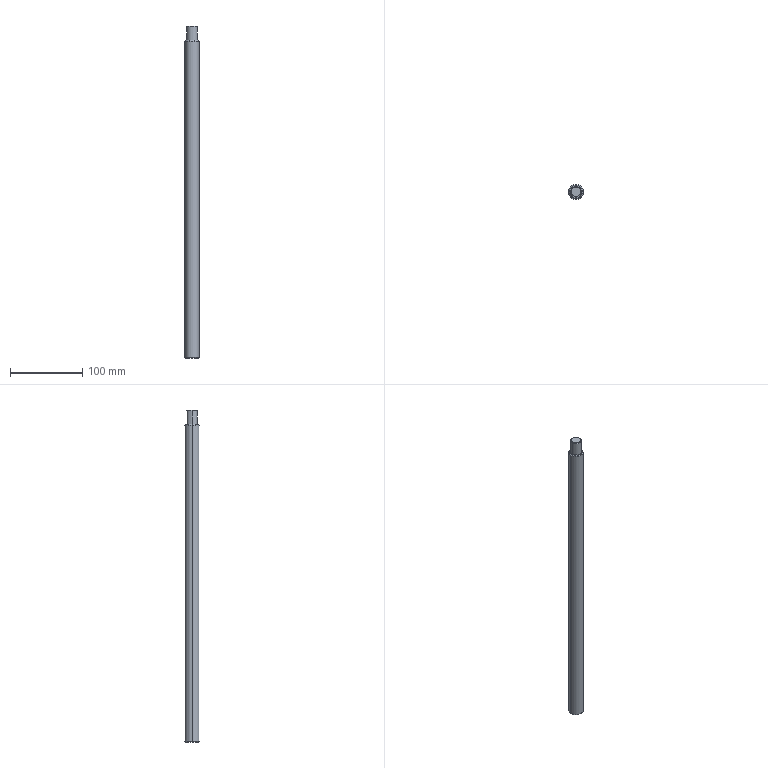Part | STEP file | 1 solid | 13 faces | box 20 x 20 x 460 mm | volume 141681 mm3 | cone 6 | cylinder 4 | plane 3 | commonest cylinder face diameters 15 x2 20 x2
STEP:
#1=CARTESIAN_POINT('',(0.,0.,0.));
#2=DIRECTION('',(0.,0.,1.));
#3=DIRECTION('',(1.,0.,0.));
#4=AXIS2_PLACEMENT_3D('',#1,#2,#3);
#5=CARTESIAN_POINT('',(10.,0.,-229.));
#6=VERTEX_POINT('',#5);
#7=CARTESIAN_POINT('',(-10.,0.,-229.));
#8=VERTEX_POINT('',#7);
#9=CARTESIAN_POINT('',(0.,0.,-229.));
#10=DIRECTION('',(0.,0.,1.));
#11=DIRECTION('',(1.,0.,0.));
#12=AXIS2_PLACEMENT_3D('',#9,#10,#11);
#13=CIRCLE('',#12,10.);
#14=CARTESIAN_POINT('',(0.,0.,230.));
#15=DIRECTION('',(0.,0.,1.));
#16=DIRECTION('',(1.,0.,0.));
#17=AXIS2_PLACEMENT_3D('',#14,#15,#16);
#18=CYLINDRICAL_SURFACE('',#17,10.);
#19=CARTESIAN_POINT('',(0.,-459.));
#20=DIRECTION('',(1.,0.));
#21=VECTOR('',#20,1.);
#22=LINE('',#19,#21);
#23=(GEOMETRIC_REPRESENTATION_CONTEXT(2)PARAMETRIC_REPRESENTATION_CONTEXT()REPRESENTATION_CONTEXT('',''));
#24=DEFINITIONAL_REPRESENTATION('',(#22),#23);
#25=PCURVE('',#18,#24);
#26=CARTESIAN_POINT('',(0.,0.,-229.));
#27=DIRECTION('',(0.,0.,1.));
#28=DIRECTION('',(1.,0.,0.));
#29=AXIS2_PLACEMENT_3D('',#26,#27,#28);
#30=CONICAL_SURFACE('',#29,10.,0.7854);
#31=CARTESIAN_POINT('',(0.,0.));
#32=DIRECTION('',(1.,0.));
#33=VECTOR('',#32,1.);
#34=LINE('',#31,#33);
#35=(GEOMETRIC_REPRESENTATION_CONTEXT(2)PARAMETRIC_REPRESENTATION_CONTEXT()REPRESENTATION_CONTEXT('',''));
#36=DEFINITIONAL_REPRESENTATION('',(#34),#35);
#37=PCURVE('',#30,#36);
#38=SURFACE_CURVE('',#13,(#25,#37),.PCURVE_S1.);
#39=EDGE_CURVE('',#6,#8,#38,.T.);
#40=ORIENTED_EDGE('',*,*,#39,.T.);
#41=CARTESIAN_POINT('',(-10.,0.,209.));
#42=VERTEX_POINT('',#41);
#43=CARTESIAN_POINT('',(-10.,0.,230.));
#44=DIRECTION('',(0.,0.,1.));
#45=VECTOR('',#44,1.);
#46=LINE('',#43,#45);
#47=CARTESIAN_POINT('',(3.142,0.));
#48=DIRECTION('',(0.,1.));
#49=VECTOR('',#48,1.);
#50=LINE('',#47,#49);
#51=(GEOMETRIC_REPRESENTATION_CONTEXT(2)PARAMETRIC_REPRESENTATION_CONTEXT()REPRESENTATION_CONTEXT('',''));
#52=DEFINITIONAL_REPRESENTATION('',(#50),#51);
#53=PCURVE('',#18,#52);
#54=CARTESIAN_POINT('',(0.,0.,230.));
#55=DIRECTION('',(0.,0.,1.));
#56=DIRECTION('',(1.,0.,0.));
#57=AXIS2_PLACEMENT_3D('',#54,#55,#56);
#58=CYLINDRICAL_SURFACE('',#57,10.);
#59=CARTESIAN_POINT('',(3.142,0.));
#60=DIRECTION('',(0.,1.));
#61=VECTOR('',#60,1.);
#62=LINE('',#59,#61);
#63=(GEOMETRIC_REPRESENTATION_CONTEXT(2)PARAMETRIC_REPRESENTATION_CONTEXT()REPRESENTATION_CONTEXT('',''));
#64=DEFINITIONAL_REPRESENTATION('',(#62),#63);
#65=PCURVE('',#58,#64);
#66=SURFACE_CURVE('',#46,(#53,#65),.PCURVE_S1.);
#67=EDGE_CURVE('',#8,#42,#66,.T.);
#68=ORIENTED_EDGE('',*,*,#67,.T.);
#69=CARTESIAN_POINT('',(10.,0.,209.));
#70=VERTEX_POINT('',#69);
#71=CARTESIAN_POINT('',(0.,0.,209.));
#72=DIRECTION('',(0.,0.,-1.));
#73=DIRECTION('',(1.,0.,0.));
#74=AXIS2_PLACEMENT_3D('',#71,#72,#73);
#75=CIRCLE('',#74,10.);
#76=CARTESIAN_POINT('',(6.283,-21.));
#77=DIRECTION('',(-1.,0.));
#78=VECTOR('',#77,1.);
#79=LINE('',#76,#78);
#80=(GEOMETRIC_REPRESENTATION_CONTEXT(2)PARAMETRIC_REPRESENTATION_CONTEXT()REPRESENTATION_CONTEXT('',''));
#81=DEFINITIONAL_REPRESENTATION('',(#79),#80);
#82=PCURVE('',#18,#81);
#83=CARTESIAN_POINT('',(0.,0.,209.));
#84=DIRECTION('',(0.,0.,-1.));
#85=DIRECTION('',(-1.,0.,0.));
#86=AXIS2_PLACEMENT_3D('',#83,#84,#85);
#87=CONICAL_SURFACE('',#86,10.,0.7854);
#88=CARTESIAN_POINT('',(-3.142,0.));
#89=DIRECTION('',(1.,0.));
#90=VECTOR('',#89,1.);
#91=LINE('',#88,#90);
#92=(GEOMETRIC_REPRESENTATION_CONTEXT(2)PARAMETRIC_REPRESENTATION_CONTEXT()REPRESENTATION_CONTEXT('',''));
#93=DEFINITIONAL_REPRESENTATION('',(#91),#92);
#94=PCURVE('',#87,#93);
#95=SURFACE_CURVE('',#75,(#82,#94),.PCURVE_S1.);
#96=EDGE_CURVE('',#42,#70,#95,.T.);
#97=ORIENTED_EDGE('',*,*,#96,.T.);
#98=CARTESIAN_POINT('',(10.,0.,230.));
#99=DIRECTION('',(0.,0.,1.));
#100=VECTOR('',#99,1.);
#101=LINE('',#98,#100);
#102=CARTESIAN_POINT('',(0.,0.));
#103=DIRECTION('',(0.,1.));
#104=VECTOR('',#103,1.);
#105=LINE('',#102,#104);
#106=(GEOMETRIC_REPRESENTATION_CONTEXT(2)PARAMETRIC_REPRESENTATION_CONTEXT()REPRESENTATION_CONTEXT('',''));
#107=DEFINITIONAL_REPRESENTATION('',(#105),#106);
#108=PCURVE('',#18,#107);
#109=CARTESIAN_POINT('',(6.283,0.));
#110=DIRECTION('',(0.,1.));
#111=VECTOR('',#110,1.);
#112=LINE('',#109,#111);
#113=(GEOMETRIC_REPRESENTATION_CONTEXT(2)PARAMETRIC_REPRESENTATION_CONTEXT()REPRESENTATION_CONTEXT('',''));
#114=DEFINITIONAL_REPRESENTATION('',(#112),#113);
#115=PCURVE('',#58,#114);
#116=SURFACE_CURVE('',#101,(#108,#115),.PCURVE_S1.);
#117=EDGE_CURVE('',#6,#70,#116,.T.);
#118=ORIENTED_EDGE('',*,*,#117,.F.);
#119=EDGE_LOOP('',(#40,#68,#97,#118));
#120=FACE_BOUND('',#119,.T.);
#121=ADVANCED_FACE('',(#120),#18,.T.);
#122=CARTESIAN_POINT('',(9.,0.,-230.));
#123=VERTEX_POINT('',#122);
#124=CARTESIAN_POINT('',(-9.,0.,-230.));
#125=VERTEX_POINT('',#124);
#126=CARTESIAN_POINT('',(0.,0.,-230.));
#127=DIRECTION('',(0.,0.,1.));
#128=DIRECTION('',(1.,0.,0.));
#129=AXIS2_PLACEMENT_3D('',#126,#127,#128);
#130=CIRCLE('',#129,9.);
#131=CARTESIAN_POINT('',(0.,-1.));
#132=DIRECTION('',(1.,0.));
#133=VECTOR('',#132,1.);
#134=LINE('',#131,#133);
#135=(GEOMETRIC_REPRESENTATION_CONTEXT(2)PARAMETRIC_REPRESENTATION_CONTEXT()REPRESENTATION_CONTEXT('',''));
#136=DEFINITIONAL_REPRESENTATION('',(#134),#135);
#137=PCURVE('',#30,#136);
#138=CARTESIAN_POINT('',(0.,0.,-230.));
#139=DIRECTION('',(0.,0.,1.));
#140=DIRECTION('',(1.,0.,0.));
#141=AXIS2_PLACEMENT_3D('',#138,#139,#140);
#142=PLANE('',#141);
#143=CARTESIAN_POINT('',(0.,0.));
#144=DIRECTION('',(1.,0.));
#145=AXIS2_PLACEMENT_2D('',#143,#144);
#146=CIRCLE('',#145,9.);
#147=(GEOMETRIC_REPRESENTATION_CONTEXT(2)PARAMETRIC_REPRESENTATION_CONTEXT()REPRESENTATION_CONTEXT('',''));
#148=DEFINITIONAL_REPRESENTATION('',(#146),#147);
#149=PCURVE('',#142,#148);
#150=SURFACE_CURVE('',#130,(#137,#149),.PCURVE_S1.);
#151=EDGE_CURVE('',#123,#125,#150,.T.);
#152=ORIENTED_EDGE('',*,*,#151,.T.);
#153=CARTESIAN_POINT('',(-10.,0.,-229.));
#154=DIRECTION('',(-0.7071,0.,0.7071));
#155=VECTOR('',#154,1.);
#156=LINE('',#153,#155);
#157=CARTESIAN_POINT('',(3.142,0.));
#158=DIRECTION('',(0.,1.));
#159=VECTOR('',#158,1.);
#160=LINE('',#157,#159);
#161=(GEOMETRIC_REPRESENTATION_CONTEXT(2)PARAMETRIC_REPRESENTATION_CONTEXT()REPRESENTATION_CONTEXT('',''));
#162=DEFINITIONAL_REPRESENTATION('',(#160),#161);
#163=PCURVE('',#30,#162);
#164=CARTESIAN_POINT('',(0.,0.,-229.));
#165=DIRECTION('',(0.,0.,1.));
#166=DIRECTION('',(1.,0.,0.));
#167=AXIS2_PLACEMENT_3D('',#164,#165,#166);
#168=CONICAL_SURFACE('',#167,10.,0.7854);
#169=CARTESIAN_POINT('',(3.142,0.));
#170=DIRECTION('',(0.,1.));
#171=VECTOR('',#170,1.);
#172=LINE('',#169,#171);
#173=(GEOMETRIC_REPRESENTATION_CONTEXT(2)PARAMETRIC_REPRESENTATION_CONTEXT()REPRESENTATION_CONTEXT('',''));
#174=DEFINITIONAL_REPRESENTATION('',(#172),#173);
#175=PCURVE('',#168,#174);
#176=SURFACE_CURVE('',#156,(#163,#175),.PCURVE_S1.);
#177=EDGE_CURVE('',#125,#8,#176,.T.);
#178=ORIENTED_EDGE('',*,*,#177,.T.);
#179=ORIENTED_EDGE('',*,*,#39,.F.);
#180=CARTESIAN_POINT('',(10.,0.,-229.));
#181=DIRECTION('',(0.7071,0.,0.7071));
#182=VECTOR('',#181,1.);
#183=LINE('',#180,#182);
#184=CARTESIAN_POINT('',(0.,0.));
#185=DIRECTION('',(0.,1.));
#186=VECTOR('',#185,1.);
#187=LINE('',#184,#186);
#188=(GEOMETRIC_REPRESENTATION_CONTEXT(2)PARAMETRIC_REPRESENTATION_CONTEXT()REPRESENTATION_CONTEXT('',''));
#189=DEFINITIONAL_REPRESENTATION('',(#187),#188);
#190=PCURVE('',#30,#189);
#191=CARTESIAN_POINT('',(6.283,0.));
#192=DIRECTION('',(0.,1.));
#193=VECTOR('',#192,1.);
#194=LINE('',#191,#193);
#195=(GEOMETRIC_REPRESENTATION_CONTEXT(2)PARAMETRIC_REPRESENTATION_CONTEXT()REPRESENTATION_CONTEXT('',''));
#196=DEFINITIONAL_REPRESENTATION('',(#194),#195);
#197=PCURVE('',#168,#196);
#198=SURFACE_CURVE('',#183,(#190,#197),.PCURVE_S1.);
#199=EDGE_CURVE('',#123,#6,#198,.T.);
#200=ORIENTED_EDGE('',*,*,#199,.F.);
#201=EDGE_LOOP('',(#152,#178,#179,#200));
#202=FACE_BOUND('',#201,.T.);
#203=ADVANCED_FACE('',(#202),#30,.T.);
#204=CARTESIAN_POINT('',(-9.,0.,210.));
#205=VERTEX_POINT('',#204);
#206=CARTESIAN_POINT('',(9.,0.,210.));
#207=VERTEX_POINT('',#206);
#208=CARTESIAN_POINT('',(0.,0.,210.));
#209=DIRECTION('',(0.,0.,-1.));
#210=DIRECTION('',(-1.,0.,0.));
#211=AXIS2_PLACEMENT_3D('',#208,#209,#210);
#212=CIRCLE('',#211,9.);
#213=CARTESIAN_POINT('',(0.,-1.));
#214=DIRECTION('',(1.,0.));
#215=VECTOR('',#214,1.);
#216=LINE('',#213,#215);
#217=(GEOMETRIC_REPRESENTATION_CONTEXT(2)PARAMETRIC_REPRESENTATION_CONTEXT()REPRESENTATION_CONTEXT('',''));
#218=DEFINITIONAL_REPRESENTATION('',(#216),#217);
#219=PCURVE('',#87,#218);
#220=CARTESIAN_POINT('',(0.,0.,210.));
#221=DIRECTION('',(0.,0.,1.));
#222=DIRECTION('',(1.,0.,0.));
#223=AXIS2_PLACEMENT_3D('',#220,#221,#222);
#224=PLANE('',#223);
#225=CARTESIAN_POINT('',(-9.,0.));
#226=CARTESIAN_POINT('',(-9.,15.588));
#227=CARTESIAN_POINT('',(4.5,7.794));
#228=CARTESIAN_POINT('',(18.,0.));
#229=CARTESIAN_POINT('',(4.5,-7.794));
#230=CARTESIAN_POINT('',(-9.,-15.588));
#231=CARTESIAN_POINT('',(-9.,0.));
#232=(BOUNDED_CURVE()B_SPLINE_CURVE(2,(#225,#226,#227,#228,#229,#230,#231),.UNSPECIFIED.,.T.,.F.)B_SPLINE_CURVE_WITH_KNOTS((1,2,2,2,2,1),(-2.094,0.,2.094,4.189,6.283,8.378),.UNSPECIFIED.)CURVE()GEOMETRIC_REPRESENTATION_ITEM()RATIONAL_B_SPLINE_CURVE((1.,0.5,1.,0.5,1.,0.5,1.))REPRESENTATION_ITEM(''));
#233=(GEOMETRIC_REPRESENTATION_CONTEXT(2)PARAMETRIC_REPRESENTATION_CONTEXT()REPRESENTATION_CONTEXT('',''));
#234=DEFINITIONAL_REPRESENTATION('',(#232),#233);
#235=PCURVE('',#224,#234);
#236=SURFACE_CURVE('',#212,(#219,#235),.PCURVE_S1.);
#237=EDGE_CURVE('',#205,#207,#236,.T.);
#238=ORIENTED_EDGE('',*,*,#237,.T.);
#239=CARTESIAN_POINT('',(10.,0.,209.));
#240=DIRECTION('',(0.7071,0.,-0.7071));
#241=VECTOR('',#240,1.);
#242=LINE('',#239,#241);
#243=CARTESIAN_POINT('',(3.142,0.));
#244=DIRECTION('',(0.,1.));
#245=VECTOR('',#244,1.);
#246=LINE('',#243,#245);
#247=(GEOMETRIC_REPRESENTATION_CONTEXT(2)PARAMETRIC_REPRESENTATION_CONTEXT()REPRESENTATION_CONTEXT('',''));
#248=DEFINITIONAL_REPRESENTATION('',(#246),#247);
#249=PCURVE('',#87,#248);
#250=CARTESIAN_POINT('',(0.,0.,209.));
#251=DIRECTION('',(0.,0.,-1.));
#252=DIRECTION('',(-1.,0.,0.));
#253=AXIS2_PLACEMENT_3D('',#250,#251,#252);
#254=CONICAL_SURFACE('',#253,10.,0.7854);
#255=CARTESIAN_POINT('',(3.142,0.));
#256=DIRECTION('',(0.,1.));
#257=VECTOR('',#256,1.);
#258=LINE('',#255,#257);
#259=(GEOMETRIC_REPRESENTATION_CONTEXT(2)PARAMETRIC_REPRESENTATION_CONTEXT()REPRESENTATION_CONTEXT('',''));
#260=DEFINITIONAL_REPRESENTATION('',(#258),#259);
#261=PCURVE('',#254,#260);
#262=SURFACE_CURVE('',#242,(#249,#261),.PCURVE_S1.);
#263=EDGE_CURVE('',#207,#70,#262,.T.);
#264=ORIENTED_EDGE('',*,*,#263,.T.);
#265=ORIENTED_EDGE('',*,*,#96,.F.);
#266=CARTESIAN_POINT('',(-10.,0.,209.));
#267=DIRECTION('',(-0.7071,0.,-0.7071));
#268=VECTOR('',#267,1.);
#269=LINE('',#266,#268);
#270=CARTESIAN_POINT('',(0.,0.));
#271=DIRECTION('',(0.,1.));
#272=VECTOR('',#271,1.);
#273=LINE('',#270,#272);
#274=(GEOMETRIC_REPRESENTATION_CONTEXT(2)PARAMETRIC_REPRESENTATION_CONTEXT()REPRESENTATION_CONTEXT('',''));
#275=DEFINITIONAL_REPRESENTATION('',(#273),#274);
#276=PCURVE('',#87,#275);
#277=CARTESIAN_POINT('',(6.283,0.));
#278=DIRECTION('',(0.,1.));
#279=VECTOR('',#278,1.);
#280=LINE('',#277,#279);
#281=(GEOMETRIC_REPRESENTATION_CONTEXT(2)PARAMETRIC_REPRESENTATION_CONTEXT()REPRESENTATION_CONTEXT('',''));
#282=DEFINITIONAL_REPRESENTATION('',(#280),#281);
#283=PCURVE('',#254,#282);
#284=SURFACE_CURVE('',#269,(#276,#283),.PCURVE_S1.);
#285=EDGE_CURVE('',#205,#42,#284,.T.);
#286=ORIENTED_EDGE('',*,*,#285,.F.);
#287=EDGE_LOOP('',(#238,#264,#265,#286));
#288=FACE_BOUND('',#287,.T.);
#289=ADVANCED_FACE('',(#288),#87,.T.);
#290=CARTESIAN_POINT('',(-7.5,0.,229.));
#291=VERTEX_POINT('',#290);
#292=CARTESIAN_POINT('',(7.5,0.,229.));
#293=VERTEX_POINT('',#292);
#294=CARTESIAN_POINT('',(0.,0.,229.));
#295=DIRECTION('',(0.,0.,-1.));
#296=DIRECTION('',(-1.,0.,0.));
#297=AXIS2_PLACEMENT_3D('',#294,#295,#296);
#298=CIRCLE('',#297,7.5);
#299=CARTESIAN_POINT('',(0.,0.,210.));
#300=DIRECTION('',(0.,0.,-1.));
#301=DIRECTION('',(-1.,0.,0.));
#302=AXIS2_PLACEMENT_3D('',#299,#300,#301);
#303=CYLINDRICAL_SURFACE('',#302,7.5);
#304=CARTESIAN_POINT('',(0.,-19.));
#305=DIRECTION('',(1.,0.));
#306=VECTOR('',#305,1.);
#307=LINE('',#304,#306);
#308=(GEOMETRIC_REPRESENTATION_CONTEXT(2)PARAMETRIC_REPRESENTATION_CONTEXT()REPRESENTATION_CONTEXT('',''));
#309=DEFINITIONAL_REPRESENTATION('',(#307),#308);
#310=PCURVE('',#303,#309);
#311=CARTESIAN_POINT('',(0.,0.,229.));
#312=DIRECTION('',(0.,0.,-1.));
#313=DIRECTION('',(-1.,0.,0.));
#314=AXIS2_PLACEMENT_3D('',#311,#312,#313);
#315=CONICAL_SURFACE('',#314,7.5,0.7854);
#316=CARTESIAN_POINT('',(0.,0.));
#317=DIRECTION('',(1.,0.));
#318=VECTOR('',#317,1.);
#319=LINE('',#316,#318);
#320=(GEOMETRIC_REPRESENTATION_CONTEXT(2)PARAMETRIC_REPRESENTATION_CONTEXT()REPRESENTATION_CONTEXT('',''));
#321=DEFINITIONAL_REPRESENTATION('',(#319),#320);
#322=PCURVE('',#315,#321);
#323=SURFACE_CURVE('',#298,(#310,#322),.PCURVE_S1.);
#324=EDGE_CURVE('',#291,#293,#323,.T.);
#325=ORIENTED_EDGE('',*,*,#324,.T.);
#326=CARTESIAN_POINT('',(7.5,0.,210.));
#327=VERTEX_POINT('',#326);
#328=CARTESIAN_POINT('',(7.5,0.,210.));
#329=DIRECTION('',(0.,0.,-1.));
#330=VECTOR('',#329,1.);
#331=LINE('',#328,#330);
#332=CARTESIAN_POINT('',(3.142,0.));
#333=DIRECTION('',(0.,1.));
#334=VECTOR('',#333,1.);
#335=LINE('',#332,#334);
#336=(GEOMETRIC_REPRESENTATION_CONTEXT(2)PARAMETRIC_REPRESENTATION_CONTEXT()REPRESENTATION_CONTEXT('',''));
#337=DEFINITIONAL_REPRESENTATION('',(#335),#336);
#338=PCURVE('',#303,#337);
#339=CARTESIAN_POINT('',(0.,0.,210.));
#340=DIRECTION('',(0.,0.,-1.));
#341=DIRECTION('',(-1.,0.,0.));
#342=AXIS2_PLACEMENT_3D('',#339,#340,#341);
#343=CYLINDRICAL_SURFACE('',#342,7.5);
#344=CARTESIAN_POINT('',(3.142,0.));
#345=DIRECTION('',(0.,1.));
#346=VECTOR('',#345,1.);
#347=LINE('',#344,#346);
#348=(GEOMETRIC_REPRESENTATION_CONTEXT(2)PARAMETRIC_REPRESENTATION_CONTEXT()REPRESENTATION_CONTEXT('',''));
#349=DEFINITIONAL_REPRESENTATION('',(#347),#348);
#350=PCURVE('',#343,#349);
#351=SURFACE_CURVE('',#331,(#338,#350),.PCURVE_S1.);
#352=EDGE_CURVE('',#293,#327,#351,.T.);
#353=ORIENTED_EDGE('',*,*,#352,.T.);
#354=CARTESIAN_POINT('',(-7.5,0.,210.));
#355=VERTEX_POINT('',#354);
#356=CARTESIAN_POINT('',(0.,0.,210.));
#357=DIRECTION('',(0.,0.,-1.));
#358=DIRECTION('',(-1.,0.,0.));
#359=AXIS2_PLACEMENT_3D('',#356,#357,#358);
#360=CIRCLE('',#359,7.5);
#361=CARTESIAN_POINT('',(0.,0.));
#362=DIRECTION('',(1.,0.));
#363=VECTOR('',#362,1.);
#364=LINE('',#361,#363);
#365=(GEOMETRIC_REPRESENTATION_CONTEXT(2)PARAMETRIC_REPRESENTATION_CONTEXT()REPRESENTATION_CONTEXT('',''));
#366=DEFINITIONAL_REPRESENTATION('',(#364),#365);
#367=PCURVE('',#303,#366);
#368=CARTESIAN_POINT('',(-7.5,0.));
#369=CARTESIAN_POINT('',(-7.5,12.99));
#370=CARTESIAN_POINT('',(3.75,6.495));
#371=CARTESIAN_POINT('',(15.,0.));
#372=CARTESIAN_POINT('',(3.75,-6.495));
#373=CARTESIAN_POINT('',(-7.5,-12.99));
#374=CARTESIAN_POINT('',(-7.5,0.));
#375=(BOUNDED_CURVE()B_SPLINE_CURVE(2,(#368,#369,#370,#371,#372,#373,#374),.UNSPECIFIED.,.T.,.F.)B_SPLINE_CURVE_WITH_KNOTS((1,2,2,2,2,1),(-2.094,0.,2.094,4.189,6.283,8.378),.UNSPECIFIED.)CURVE()GEOMETRIC_REPRESENTATION_ITEM()RATIONAL_B_SPLINE_CURVE((1.,0.5,1.,0.5,1.,0.5,1.))REPRESENTATION_ITEM(''));
#376=(GEOMETRIC_REPRESENTATION_CONTEXT(2)PARAMETRIC_REPRESENTATION_CONTEXT()REPRESENTATION_CONTEXT('',''));
#377=DEFINITIONAL_REPRESENTATION('',(#375),#376);
#378=PCURVE('',#224,#377);
#379=SURFACE_CURVE('',#360,(#367,#378),.PCURVE_S1.);
#380=EDGE_CURVE('',#355,#327,#379,.T.);
#381=ORIENTED_EDGE('',*,*,#380,.F.);
#382=CARTESIAN_POINT('',(-7.5,0.,210.));
#383=DIRECTION('',(0.,0.,-1.));
#384=VECTOR('',#383,1.);
#385=LINE('',#382,#384);
#386=CARTESIAN_POINT('',(0.,0.));
#387=DIRECTION('',(0.,1.));
#388=VECTOR('',#387,1.);
#389=LINE('',#386,#388);
#390=(GEOMETRIC_REPRESENTATION_CONTEXT(2)PARAMETRIC_REPRESENTATION_CONTEXT()REPRESENTATION_CONTEXT('',''));
#391=DEFINITIONAL_REPRESENTATION('',(#389),#390);
#392=PCURVE('',#303,#391);
#393=CARTESIAN_POINT('',(6.283,0.));
#394=DIRECTION('',(0.,1.));
#395=VECTOR('',#394,1.);
#396=LINE('',#393,#395);
#397=(GEOMETRIC_REPRESENTATION_CONTEXT(2)PARAMETRIC_REPRESENTATION_CONTEXT()REPRESENTATION_CONTEXT('',''));
#398=DEFINITIONAL_REPRESENTATION('',(#396),#397);
#399=PCURVE('',#343,#398);
#400=SURFACE_CURVE('',#385,(#392,#399),.PCURVE_S1.);
#401=EDGE_CURVE('',#291,#355,#400,.T.);
#402=ORIENTED_EDGE('',*,*,#401,.F.);
#403=EDGE_LOOP('',(#325,#353,#381,#402));
#404=FACE_BOUND('',#403,.T.);
#405=ADVANCED_FACE('',(#404),#303,.T.);
#406=CARTESIAN_POINT('',(-6.5,0.,230.));
#407=VERTEX_POINT('',#406);
#408=CARTESIAN_POINT('',(6.5,0.,230.));
#409=VERTEX_POINT('',#408);
#410=CARTESIAN_POINT('',(0.,0.,230.));
#411=DIRECTION('',(0.,0.,-1.));
#412=DIRECTION('',(-1.,0.,0.));
#413=AXIS2_PLACEMENT_3D('',#410,#411,#412);
#414=CIRCLE('',#413,6.5);
#415=CARTESIAN_POINT('',(0.,-1.));
#416=DIRECTION('',(1.,0.));
#417=VECTOR('',#416,1.);
#418=LINE('',#415,#417);
#419=(GEOMETRIC_REPRESENTATION_CONTEXT(2)PARAMETRIC_REPRESENTATION_CONTEXT()REPRESENTATION_CONTEXT('',''));
#420=DEFINITIONAL_REPRESENTATION('',(#418),#419);
#421=PCURVE('',#315,#420);
#422=CARTESIAN_POINT('',(0.,0.,230.));
#423=DIRECTION('',(0.,0.,1.));
#424=DIRECTION('',(1.,0.,0.));
#425=AXIS2_PLACEMENT_3D('',#422,#423,#424);
#426=PLANE('',#425);
#427=CARTESIAN_POINT('',(-6.5,0.));
#428=CARTESIAN_POINT('',(-6.5,11.258));
#429=CARTESIAN_POINT('',(3.25,5.629));
#430=CARTESIAN_POINT('',(13.,0.));
#431=CARTESIAN_POINT('',(3.25,-5.629));
#432=CARTESIAN_POINT('',(-6.5,-11.258));
#433=CARTESIAN_POINT('',(-6.5,0.));
#434=(BOUNDED_CURVE()B_SPLINE_CURVE(2,(#427,#428,#429,#430,#431,#432,#433),.UNSPECIFIED.,.T.,.F.)B_SPLINE_CURVE_WITH_KNOTS((1,2,2,2,2,1),(-2.094,0.,2.094,4.189,6.283,8.378),.UNSPECIFIED.)CURVE()GEOMETRIC_REPRESENTATION_ITEM()RATIONAL_B_SPLINE_CURVE((1.,0.5,1.,0.5,1.,0.5,1.))REPRESENTATION_ITEM(''));
#435=(GEOMETRIC_REPRESENTATION_CONTEXT(2)PARAMETRIC_REPRESENTATION_CONTEXT()REPRESENTATION_CONTEXT('',''));
#436=DEFINITIONAL_REPRESENTATION('',(#434),#435);
#437=PCURVE('',#426,#436);
#438=SURFACE_CURVE('',#414,(#421,#437),.PCURVE_S1.);
#439=EDGE_CURVE('',#407,#409,#438,.T.);
#440=ORIENTED_EDGE('',*,*,#439,.T.);
#441=CARTESIAN_POINT('',(7.5,0.,229.));
#442=DIRECTION('',(0.7071,0.,-0.7071));
#443=VECTOR('',#442,1.);
#444=LINE('',#441,#443);
#445=CARTESIAN_POINT('',(3.142,0.));
#446=DIRECTION('',(0.,1.));
#447=VECTOR('',#446,1.);
#448=LINE('',#445,#447);
#449=(GEOMETRIC_REPRESENTATION_CONTEXT(2)PARAMETRIC_REPRESENTATION_CONTEXT()REPRESENTATION_CONTEXT('',''));
#450=DEFINITIONAL_REPRESENTATION('',(#448),#449);
#451=PCURVE('',#315,#450);
#452=CARTESIAN_POINT('',(0.,0.,229.));
#453=DIRECTION('',(0.,0.,-1.));
#454=DIRECTION('',(-1.,0.,0.));
#455=AXIS2_PLACEMENT_3D('',#452,#453,#454);
#456=CONICAL_SURFACE('',#455,7.5,0.7854);
#457=CARTESIAN_POINT('',(3.142,0.));
#458=DIRECTION('',(0.,1.));
#459=VECTOR('',#458,1.);
#460=LINE('',#457,#459);
#461=(GEOMETRIC_REPRESENTATION_CONTEXT(2)PARAMETRIC_REPRESENTATION_CONTEXT()REPRESENTATION_CONTEXT('',''));
#462=DEFINITIONAL_REPRESENTATION('',(#460),#461);
#463=PCURVE('',#456,#462);
#464=SURFACE_CURVE('',#444,(#451,#463),.PCURVE_S1.);
#465=EDGE_CURVE('',#409,#293,#464,.T.);
#466=ORIENTED_EDGE('',*,*,#465,.T.);
#467=ORIENTED_EDGE('',*,*,#324,.F.);
#468=CARTESIAN_POINT('',(-7.5,0.,229.));
#469=DIRECTION('',(-0.7071,0.,-0.7071));
#470=VECTOR('',#469,1.);
#471=LINE('',#468,#470);
#472=CARTESIAN_POINT('',(0.,0.));
#473=DIRECTION('',(0.,1.));
#474=VECTOR('',#473,1.);
#475=LINE('',#472,#474);
#476=(GEOMETRIC_REPRESENTATION_CONTEXT(2)PARAMETRIC_REPRESENTATION_CONTEXT()REPRESENTATION_CONTEXT('',''));
#477=DEFINITIONAL_REPRESENTATION('',(#475),#476);
#478=PCURVE('',#315,#477);
#479=CARTESIAN_POINT('',(6.283,0.));
#480=DIRECTION('',(0.,1.));
#481=VECTOR('',#480,1.);
#482=LINE('',#479,#481);
#483=(GEOMETRIC_REPRESENTATION_CONTEXT(2)PARAMETRIC_REPRESENTATION_CONTEXT()REPRESENTATION_CONTEXT('',''));
#484=DEFINITIONAL_REPRESENTATION('',(#482),#483);
#485=PCURVE('',#456,#484);
#486=SURFACE_CURVE('',#471,(#478,#485),.PCURVE_S1.);
#487=EDGE_CURVE('',#407,#291,#486,.T.);
#488=ORIENTED_EDGE('',*,*,#487,.F.);
#489=EDGE_LOOP('',(#440,#466,#467,#488));
#490=FACE_BOUND('',#489,.T.);
#491=ADVANCED_FACE('',(#490),#315,.T.);
#492=ORIENTED_EDGE('',*,*,#67,.F.);
#493=CARTESIAN_POINT('',(0.,0.,-229.));
#494=DIRECTION('',(0.,0.,1.));
#495=DIRECTION('',(1.,0.,0.));
#496=AXIS2_PLACEMENT_3D('',#493,#494,#495);
#497=CIRCLE('',#496,10.);
#498=CARTESIAN_POINT('',(0.,-459.));
#499=DIRECTION('',(1.,0.));
#500=VECTOR('',#499,1.);
#501=LINE('',#498,#500);
#502=(GEOMETRIC_REPRESENTATION_CONTEXT(2)PARAMETRIC_REPRESENTATION_CONTEXT()REPRESENTATION_CONTEXT('',''));
#503=DEFINITIONAL_REPRESENTATION('',(#501),#502);
#504=PCURVE('',#58,#503);
#505=CARTESIAN_POINT('',(0.,0.));
#506=DIRECTION('',(1.,0.));
#507=VECTOR('',#506,1.);
#508=LINE('',#505,#507);
#509=(GEOMETRIC_REPRESENTATION_CONTEXT(2)PARAMETRIC_REPRESENTATION_CONTEXT()REPRESENTATION_CONTEXT('',''));
#510=DEFINITIONAL_REPRESENTATION('',(#508),#509);
#511=PCURVE('',#168,#510);
#512=SURFACE_CURVE('',#497,(#504,#511),.PCURVE_S1.);
#513=EDGE_CURVE('',#8,#6,#512,.T.);
#514=ORIENTED_EDGE('',*,*,#513,.T.);
#515=ORIENTED_EDGE('',*,*,#117,.T.);
#516=CARTESIAN_POINT('',(0.,0.,209.));
#517=DIRECTION('',(0.,0.,-1.));
#518=DIRECTION('',(1.,0.,0.));
#519=AXIS2_PLACEMENT_3D('',#516,#517,#518);
#520=CIRCLE('',#519,10.);
#521=CARTESIAN_POINT('',(6.283,-21.));
#522=DIRECTION('',(-1.,0.));
#523=VECTOR('',#522,1.);
#524=LINE('',#521,#523);
#525=(GEOMETRIC_REPRESENTATION_CONTEXT(2)PARAMETRIC_REPRESENTATION_CONTEXT()REPRESENTATION_CONTEXT('',''));
#526=DEFINITIONAL_REPRESENTATION('',(#524),#525);
#527=PCURVE('',#58,#526);
#528=CARTESIAN_POINT('',(3.142,0.));
#529=DIRECTION('',(1.,0.));
#530=VECTOR('',#529,1.);
#531=LINE('',#528,#530);
#532=(GEOMETRIC_REPRESENTATION_CONTEXT(2)PARAMETRIC_REPRESENTATION_CONTEXT()REPRESENTATION_CONTEXT('',''));
#533=DEFINITIONAL_REPRESENTATION('',(#531),#532);
#534=PCURVE('',#254,#533);
#535=SURFACE_CURVE('',#520,(#527,#534),.PCURVE_S1.);
#536=EDGE_CURVE('',#70,#42,#535,.T.);
#537=ORIENTED_EDGE('',*,*,#536,.T.);
#538=EDGE_LOOP('',(#492,#514,#515,#537));
#539=FACE_BOUND('',#538,.T.);
#540=ADVANCED_FACE('',(#539),#58,.T.);
#541=ORIENTED_EDGE('',*,*,#177,.F.);
#542=CARTESIAN_POINT('',(0.,0.,-230.));
#543=DIRECTION('',(0.,0.,1.));
#544=DIRECTION('',(1.,0.,0.));
#545=AXIS2_PLACEMENT_3D('',#542,#543,#544);
#546=CIRCLE('',#545,9.);
#547=CARTESIAN_POINT('',(0.,-1.));
#548=DIRECTION('',(1.,0.));
#549=VECTOR('',#548,1.);
#550=LINE('',#547,#549);
#551=(GEOMETRIC_REPRESENTATION_CONTEXT(2)PARAMETRIC_REPRESENTATION_CONTEXT()REPRESENTATION_CONTEXT('',''));
#552=DEFINITIONAL_REPRESENTATION('',(#550),#551);
#553=PCURVE('',#168,#552);
#554=CARTESIAN_POINT('',(0.,0.));
#555=DIRECTION('',(1.,0.));
#556=AXIS2_PLACEMENT_2D('',#554,#555);
#557=CIRCLE('',#556,9.);
#558=(GEOMETRIC_REPRESENTATION_CONTEXT(2)PARAMETRIC_REPRESENTATION_CONTEXT()REPRESENTATION_CONTEXT('',''));
#559=DEFINITIONAL_REPRESENTATION('',(#557),#558);
#560=PCURVE('',#142,#559);
#561=SURFACE_CURVE('',#546,(#553,#560),.PCURVE_S1.);
#562=EDGE_CURVE('',#125,#123,#561,.T.);
#563=ORIENTED_EDGE('',*,*,#562,.T.);
#564=ORIENTED_EDGE('',*,*,#199,.T.);
#565=ORIENTED_EDGE('',*,*,#513,.F.);
#566=EDGE_LOOP('',(#541,#563,#564,#565));
#567=FACE_BOUND('',#566,.T.);
#568=ADVANCED_FACE('',(#567),#168,.T.);
#569=ORIENTED_EDGE('',*,*,#263,.F.);
#570=CARTESIAN_POINT('',(0.,0.,210.));
#571=DIRECTION('',(0.,0.,-1.));
#572=DIRECTION('',(-1.,0.,0.));
#573=AXIS2_PLACEMENT_3D('',#570,#571,#572);
#574=CIRCLE('',#573,9.);
#575=CARTESIAN_POINT('',(0.,-1.));
#576=DIRECTION('',(1.,0.));
#577=VECTOR('',#576,1.);
#578=LINE('',#575,#577);
#579=(GEOMETRIC_REPRESENTATION_CONTEXT(2)PARAMETRIC_REPRESENTATION_CONTEXT()REPRESENTATION_CONTEXT('',''));
#580=DEFINITIONAL_REPRESENTATION('',(#578),#579);
#581=PCURVE('',#254,#580);
#582=CARTESIAN_POINT('',(-9.,0.));
#583=CARTESIAN_POINT('',(-9.,15.588));
#584=CARTESIAN_POINT('',(4.5,7.794));
#585=CARTESIAN_POINT('',(18.,0.));
#586=CARTESIAN_POINT('',(4.5,-7.794));
#587=CARTESIAN_POINT('',(-9.,-15.588));
#588=CARTESIAN_POINT('',(-9.,0.));
#589=(BOUNDED_CURVE()B_SPLINE_CURVE(2,(#582,#583,#584,#585,#586,#587,#588),.UNSPECIFIED.,.T.,.F.)B_SPLINE_CURVE_WITH_KNOTS((1,2,2,2,2,1),(-2.094,0.,2.094,4.189,6.283,8.378),.UNSPECIFIED.)CURVE()GEOMETRIC_REPRESENTATION_ITEM()RATIONAL_B_SPLINE_CURVE((1.,0.5,1.,0.5,1.,0.5,1.))REPRESENTATION_ITEM(''));
#590=(GEOMETRIC_REPRESENTATION_CONTEXT(2)PARAMETRIC_REPRESENTATION_CONTEXT()REPRESENTATION_CONTEXT('',''));
#591=DEFINITIONAL_REPRESENTATION('',(#589),#590);
#592=PCURVE('',#224,#591);
#593=SURFACE_CURVE('',#574,(#581,#592),.PCURVE_S1.);
#594=EDGE_CURVE('',#207,#205,#593,.T.);
#595=ORIENTED_EDGE('',*,*,#594,.T.);
#596=ORIENTED_EDGE('',*,*,#285,.T.);
#597=ORIENTED_EDGE('',*,*,#536,.F.);
#598=EDGE_LOOP('',(#569,#595,#596,#597));
#599=FACE_BOUND('',#598,.T.);
#600=ADVANCED_FACE('',(#599),#254,.T.);
#601=ORIENTED_EDGE('',*,*,#151,.F.);
#602=ORIENTED_EDGE('',*,*,#562,.F.);
#603=EDGE_LOOP('',(#601,#602));
#604=FACE_BOUND('',#603,.T.);
#605=ADVANCED_FACE('',(#604),#142,.F.);
#606=ORIENTED_EDGE('',*,*,#380,.T.);
#607=CARTESIAN_POINT('',(0.,0.,210.));
#608=DIRECTION('',(0.,0.,-1.));
#609=DIRECTION('',(-1.,0.,0.));
#610=AXIS2_PLACEMENT_3D('',#607,#608,#609);
#611=CIRCLE('',#610,7.5);
#612=CARTESIAN_POINT('',(-7.5,0.));
#613=CARTESIAN_POINT('',(-7.5,12.99));
#614=CARTESIAN_POINT('',(3.75,6.495));
#615=CARTESIAN_POINT('',(15.,0.));
#616=CARTESIAN_POINT('',(3.75,-6.495));
#617=CARTESIAN_POINT('',(-7.5,-12.99));
#618=CARTESIAN_POINT('',(-7.5,0.));
#619=(BOUNDED_CURVE()B_SPLINE_CURVE(2,(#612,#613,#614,#615,#616,#617,#618),.UNSPECIFIED.,.T.,.F.)B_SPLINE_CURVE_WITH_KNOTS((1,2,2,2,2,1),(-2.094,0.,2.094,4.189,6.283,8.378),.UNSPECIFIED.)CURVE()GEOMETRIC_REPRESENTATION_ITEM()RATIONAL_B_SPLINE_CURVE((1.,0.5,1.,0.5,1.,0.5,1.))REPRESENTATION_ITEM(''));
#620=(GEOMETRIC_REPRESENTATION_CONTEXT(2)PARAMETRIC_REPRESENTATION_CONTEXT()REPRESENTATION_CONTEXT('',''));
#621=DEFINITIONAL_REPRESENTATION('',(#619),#620);
#622=PCURVE('',#224,#621);
#623=CARTESIAN_POINT('',(0.,0.));
#624=DIRECTION('',(1.,0.));
#625=VECTOR('',#624,1.);
#626=LINE('',#623,#625);
#627=(GEOMETRIC_REPRESENTATION_CONTEXT(2)PARAMETRIC_REPRESENTATION_CONTEXT()REPRESENTATION_CONTEXT('',''));
#628=DEFINITIONAL_REPRESENTATION('',(#626),#627);
#629=PCURVE('',#343,#628);
#630=SURFACE_CURVE('',#611,(#622,#629),.PCURVE_S1.);
#631=EDGE_CURVE('',#327,#355,#630,.T.);
#632=ORIENTED_EDGE('',*,*,#631,.T.);
#633=EDGE_LOOP('',(#606,#632));
#634=FACE_BOUND('',#633,.T.);
#635=ORIENTED_EDGE('',*,*,#237,.F.);
#636=ORIENTED_EDGE('',*,*,#594,.F.);
#637=EDGE_LOOP('',(#635,#636));
#638=FACE_BOUND('',#637,.T.);
#639=ADVANCED_FACE('',(#634,#638),#224,.T.);
#640=ORIENTED_EDGE('',*,*,#352,.F.);
#641=CARTESIAN_POINT('',(0.,0.,229.));
#642=DIRECTION('',(0.,0.,-1.));
#643=DIRECTION('',(-1.,0.,0.));
#644=AXIS2_PLACEMENT_3D('',#641,#642,#643);
#645=CIRCLE('',#644,7.5);
#646=CARTESIAN_POINT('',(0.,-19.));
#647=DIRECTION('',(1.,0.));
#648=VECTOR('',#647,1.);
#649=LINE('',#646,#648);
#650=(GEOMETRIC_REPRESENTATION_CONTEXT(2)PARAMETRIC_REPRESENTATION_CONTEXT()REPRESENTATION_CONTEXT('',''));
#651=DEFINITIONAL_REPRESENTATION('',(#649),#650);
#652=PCURVE('',#343,#651);
#653=CARTESIAN_POINT('',(0.,0.));
#654=DIRECTION('',(1.,0.));
#655=VECTOR('',#654,1.);
#656=LINE('',#653,#655);
#657=(GEOMETRIC_REPRESENTATION_CONTEXT(2)PARAMETRIC_REPRESENTATION_CONTEXT()REPRESENTATION_CONTEXT('',''));
#658=DEFINITIONAL_REPRESENTATION('',(#656),#657);
#659=PCURVE('',#456,#658);
#660=SURFACE_CURVE('',#645,(#652,#659),.PCURVE_S1.);
#661=EDGE_CURVE('',#293,#291,#660,.T.);
#662=ORIENTED_EDGE('',*,*,#661,.T.);
#663=ORIENTED_EDGE('',*,*,#401,.T.);
#664=ORIENTED_EDGE('',*,*,#631,.F.);
#665=EDGE_LOOP('',(#640,#662,#663,#664));
#666=FACE_BOUND('',#665,.T.);
#667=ADVANCED_FACE('',(#666),#343,.T.);
#668=ORIENTED_EDGE('',*,*,#465,.F.);
#669=CARTESIAN_POINT('',(0.,0.,230.));
#670=DIRECTION('',(0.,0.,-1.));
#671=DIRECTION('',(-1.,0.,0.));
#672=AXIS2_PLACEMENT_3D('',#669,#670,#671);
#673=CIRCLE('',#672,6.5);
#674=CARTESIAN_POINT('',(0.,-1.));
#675=DIRECTION('',(1.,0.));
#676=VECTOR('',#675,1.);
#677=LINE('',#674,#676);
#678=(GEOMETRIC_REPRESENTATION_CONTEXT(2)PARAMETRIC_REPRESENTATION_CONTEXT()REPRESENTATION_CONTEXT('',''));
#679=DEFINITIONAL_REPRESENTATION('',(#677),#678);
#680=PCURVE('',#456,#679);
#681=CARTESIAN_POINT('',(-6.5,0.));
#682=CARTESIAN_POINT('',(-6.5,11.258));
#683=CARTESIAN_POINT('',(3.25,5.629));
#684=CARTESIAN_POINT('',(13.,0.));
#685=CARTESIAN_POINT('',(3.25,-5.629));
#686=CARTESIAN_POINT('',(-6.5,-11.258));
#687=CARTESIAN_POINT('',(-6.5,0.));
#688=(BOUNDED_CURVE()B_SPLINE_CURVE(2,(#681,#682,#683,#684,#685,#686,#687),.UNSPECIFIED.,.T.,.F.)B_SPLINE_CURVE_WITH_KNOTS((1,2,2,2,2,1),(-2.094,0.,2.094,4.189,6.283,8.378),.UNSPECIFIED.)CURVE()GEOMETRIC_REPRESENTATION_ITEM()RATIONAL_B_SPLINE_CURVE((1.,0.5,1.,0.5,1.,0.5,1.))REPRESENTATION_ITEM(''));
#689=(GEOMETRIC_REPRESENTATION_CONTEXT(2)PARAMETRIC_REPRESENTATION_CONTEXT()REPRESENTATION_CONTEXT('',''));
#690=DEFINITIONAL_REPRESENTATION('',(#688),#689);
#691=PCURVE('',#426,#690);
#692=SURFACE_CURVE('',#673,(#680,#691),.PCURVE_S1.);
#693=EDGE_CURVE('',#409,#407,#692,.T.);
#694=ORIENTED_EDGE('',*,*,#693,.T.);
#695=ORIENTED_EDGE('',*,*,#487,.T.);
#696=ORIENTED_EDGE('',*,*,#661,.F.);
#697=EDGE_LOOP('',(#668,#694,#695,#696));
#698=FACE_BOUND('',#697,.T.);
#699=ADVANCED_FACE('',(#698),#456,.T.);
#700=ORIENTED_EDGE('',*,*,#439,.F.);
#701=ORIENTED_EDGE('',*,*,#693,.F.);
#702=EDGE_LOOP('',(#700,#701));
#703=FACE_BOUND('',#702,.T.);
#704=ADVANCED_FACE('',(#703),#426,.T.);
#705=CLOSED_SHELL('',(#121,#203,#289,#405,#491,#540,#568,#600,#605,#639,#667,#699,#704));
#706=MANIFOLD_SOLID_BREP('',#705);
#707=(LENGTH_UNIT()NAMED_UNIT(*)SI_UNIT(.MILLI.,.METRE.));
#708=UNCERTAINTY_MEASURE_WITH_UNIT(LENGTH_MEASURE(0.0000001),#707,'','');
#709=(NAMED_UNIT(*)PLANE_ANGLE_UNIT()SI_UNIT($,.RADIAN.));
#710=(NAMED_UNIT(*)SI_UNIT($,.STERADIAN.)SOLID_ANGLE_UNIT());
#711=(GEOMETRIC_REPRESENTATION_CONTEXT(3)GLOBAL_UNCERTAINTY_ASSIGNED_CONTEXT((#708))GLOBAL_UNIT_ASSIGNED_CONTEXT((#707,#709,#710))REPRESENTATION_CONTEXT('',''));
#712=ADVANCED_BREP_SHAPE_REPRESENTATION('',(#4,#706),#711);